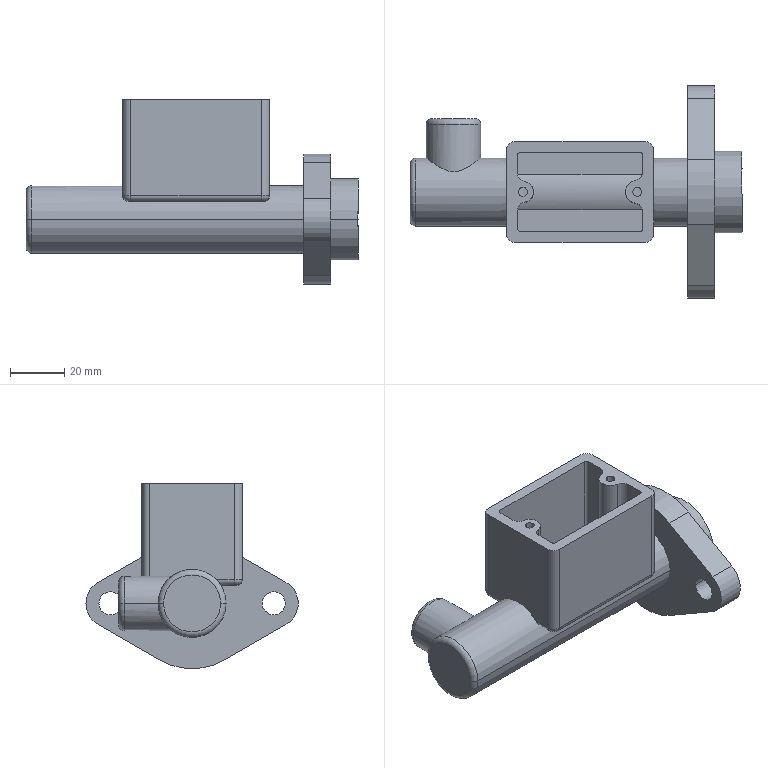Part | SolidWorks | features BaseBody 1 | 1 solid | 77 faces | box 122 x 78 x 68 mm | volume 86158 mm3 | cylinder 44 | plane 25 | torus 8 | commonest cylinder face diameters 6 x8 4 x6 8.5 x5 25 x5 2 x4 3.3 x4